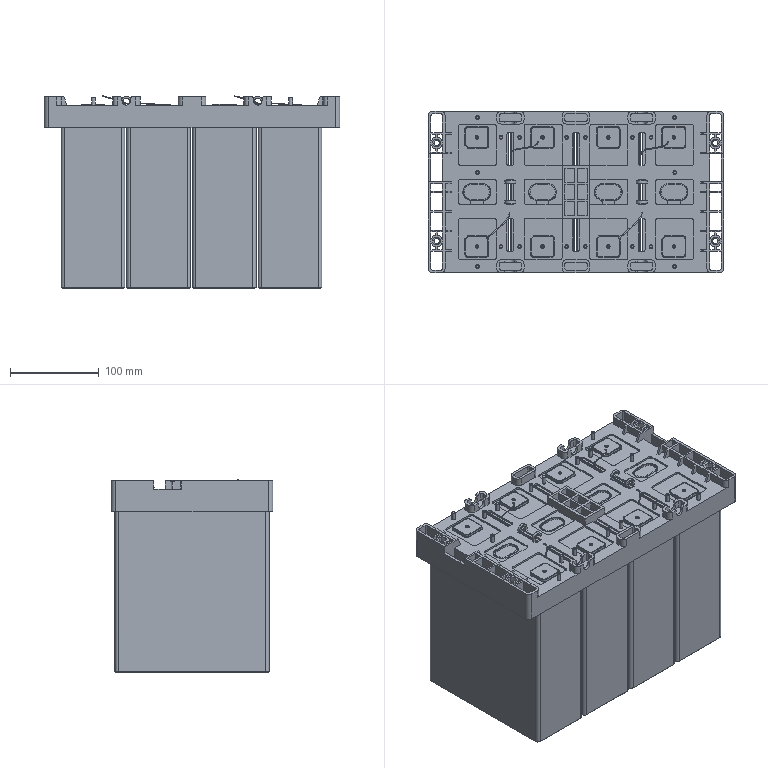Part | NX | features BREP 11 | 11 solids | 1856 faces | box 333 x 182 x 217.08 mm | volume 10398899 mm3 | plane 1202 | cylinder 554 | cone 72 | spline 24 | torus 4 | commonest cylinder face diameters 6 x148 4 x132 2 x48 10 x46 8 x28 4.22 x24